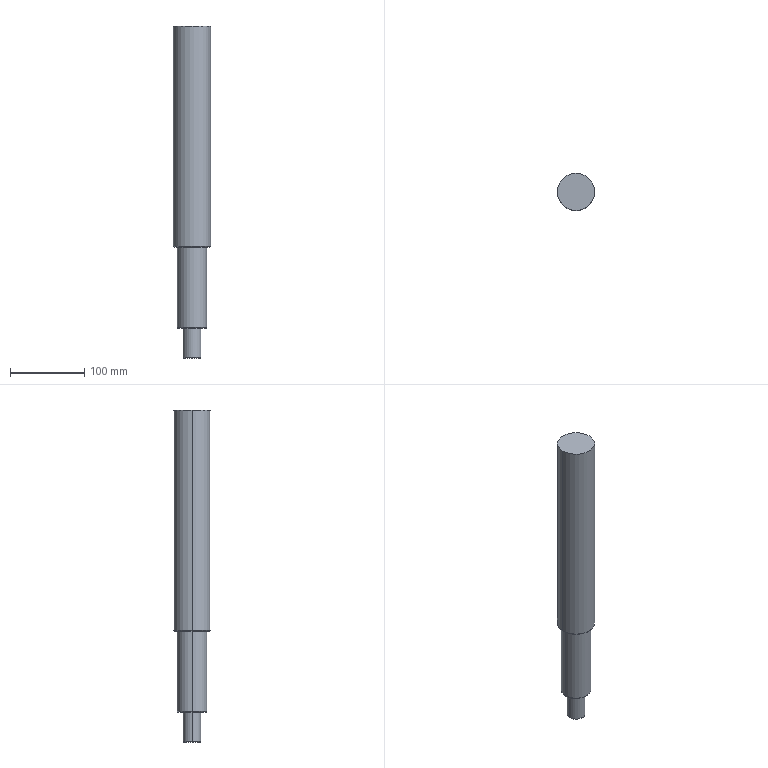Part | SolidWorks | features ICE 2, Chamfer 1, Extrusion 1 | 1 solid | 16 faces | box 50 x 50 x 446 mm | volume 738051 mm3 | cone 6 | cylinder 6 | plane 4 | commonest cylinder face diameters 24 x2 40 x2 50 x2
STEP:
#1=CARTESIAN_POINT('',(-24.,0.,-197.));
#2=VERTEX_POINT('',#1);
#3=CARTESIAN_POINT('',(24.,0.,-197.));
#4=VERTEX_POINT('',#3);
#5=CARTESIAN_POINT('',(0.,0.,-197.));
#6=DIRECTION('',(0.,0.,-1.));
#7=DIRECTION('',(-1.,0.,0.));
#8=AXIS2_PLACEMENT_3D('',#5,#6,#7);
#9=CIRCLE('',#8,24.);
#10=EDGE_CURVE('',#2,#4,#9,.T.);
#11=ORIENTED_EDGE('',*,*,#10,.F.);
#12=CARTESIAN_POINT('',(-25.,0.,-196.));
#13=VERTEX_POINT('',#12);
#14=CARTESIAN_POINT('',(-24.,0.,-197.));
#15=DIRECTION('',(-0.7071,0.,0.7071));
#16=VECTOR('',#15,1000.);
#17=LINE('',#14,#16);
#18=EDGE_CURVE('',#2,#13,#17,.T.);
#19=ORIENTED_EDGE('',*,*,#18,.T.);
#20=CARTESIAN_POINT('',(25.,0.,-196.));
#21=VERTEX_POINT('',#20);
#22=CARTESIAN_POINT('',(0.,0.,-196.));
#23=DIRECTION('',(0.,0.,1.));
#24=DIRECTION('',(-1.,0.,0.));
#25=AXIS2_PLACEMENT_3D('',#22,#23,#24);
#26=CIRCLE('',#25,25.);
#27=EDGE_CURVE('',#21,#13,#26,.T.);
#28=ORIENTED_EDGE('',*,*,#27,.F.);
#29=CARTESIAN_POINT('',(24.,0.,-197.));
#30=DIRECTION('',(0.7071,0.,0.7071));
#31=VECTOR('',#30,1000.);
#32=LINE('',#29,#31);
#33=EDGE_CURVE('',#4,#21,#32,.T.);
#34=ORIENTED_EDGE('',*,*,#33,.F.);
#35=EDGE_LOOP('',(#11,#19,#28,#34));
#36=FACE_OUTER_BOUND('',#35,.T.);
#37=CARTESIAN_POINT('',(0.,0.,-197.));
#38=DIRECTION('',(0.,0.,1.));
#39=DIRECTION('',(1.,0.,0.));
#40=AXIS2_PLACEMENT_3D('',#37,#38,#39);
#41=CONICAL_SURFACE('',#40,24.,0.7854);
#42=ADVANCED_FACE('',(#36),#41,.T.);
#43=CARTESIAN_POINT('',(-19.,0.,-306.));
#44=VERTEX_POINT('',#43);
#45=CARTESIAN_POINT('',(19.,0.,-306.));
#46=VERTEX_POINT('',#45);
#47=CARTESIAN_POINT('',(0.,0.,-306.));
#48=DIRECTION('',(0.,0.,-1.));
#49=DIRECTION('',(-1.,0.,0.));
#50=AXIS2_PLACEMENT_3D('',#47,#48,#49);
#51=CIRCLE('',#50,19.);
#52=EDGE_CURVE('',#44,#46,#51,.T.);
#53=ORIENTED_EDGE('',*,*,#52,.F.);
#54=CARTESIAN_POINT('',(-20.,0.,-305.));
#55=VERTEX_POINT('',#54);
#56=CARTESIAN_POINT('',(-20.,0.,-305.));
#57=DIRECTION('',(-0.7071,0.,0.7071));
#58=VECTOR('',#57,1000.);
#59=LINE('',#56,#58);
#60=EDGE_CURVE('',#44,#55,#59,.T.);
#61=ORIENTED_EDGE('',*,*,#60,.T.);
#62=CARTESIAN_POINT('',(20.,0.,-305.));
#63=VERTEX_POINT('',#62);
#64=CARTESIAN_POINT('',(0.,0.,-305.));
#65=DIRECTION('',(0.,0.,1.));
#66=DIRECTION('',(-1.,0.,0.));
#67=AXIS2_PLACEMENT_3D('',#64,#65,#66);
#68=CIRCLE('',#67,20.);
#69=EDGE_CURVE('',#63,#55,#68,.T.);
#70=ORIENTED_EDGE('',*,*,#69,.F.);
#71=CARTESIAN_POINT('',(20.,0.,-305.));
#72=DIRECTION('',(0.7071,0.,0.7071));
#73=VECTOR('',#72,1000.);
#74=LINE('',#71,#73);
#75=EDGE_CURVE('',#46,#63,#74,.T.);
#76=ORIENTED_EDGE('',*,*,#75,.F.);
#77=EDGE_LOOP('',(#53,#61,#70,#76));
#78=FACE_OUTER_BOUND('',#77,.T.);
#79=CARTESIAN_POINT('',(0.,0.,-305.));
#80=DIRECTION('',(0.,0.,1.));
#81=DIRECTION('',(1.,0.,0.));
#82=AXIS2_PLACEMENT_3D('',#79,#80,#81);
#83=CONICAL_SURFACE('',#82,20.,0.7854);
#84=ADVANCED_FACE('',(#78),#83,.T.);
#85=CARTESIAN_POINT('',(-11.,0.,-346.));
#86=VERTEX_POINT('',#85);
#87=CARTESIAN_POINT('',(11.,0.,-346.));
#88=VERTEX_POINT('',#87);
#89=CARTESIAN_POINT('',(0.,0.,-346.));
#90=DIRECTION('',(0.,0.,-1.));
#91=DIRECTION('',(1.,0.,0.));
#92=AXIS2_PLACEMENT_3D('',#89,#90,#91);
#93=CIRCLE('',#92,11.);
#94=EDGE_CURVE('',#86,#88,#93,.T.);
#95=ORIENTED_EDGE('',*,*,#94,.F.);
#96=CARTESIAN_POINT('',(-12.,0.,-345.));
#97=VERTEX_POINT('',#96);
#98=CARTESIAN_POINT('',(-11.,0.,-346.));
#99=DIRECTION('',(-0.7071,0.,0.7071));
#100=VECTOR('',#99,1000.);
#101=LINE('',#98,#100);
#102=EDGE_CURVE('',#86,#97,#101,.T.);
#103=ORIENTED_EDGE('',*,*,#102,.T.);
#104=CARTESIAN_POINT('',(12.,0.,-345.));
#105=VERTEX_POINT('',#104);
#106=CARTESIAN_POINT('',(0.,0.,-345.));
#107=DIRECTION('',(0.,0.,1.));
#108=DIRECTION('',(1.,0.,0.));
#109=AXIS2_PLACEMENT_3D('',#106,#107,#108);
#110=CIRCLE('',#109,12.);
#111=EDGE_CURVE('',#105,#97,#110,.T.);
#112=ORIENTED_EDGE('',*,*,#111,.F.);
#113=CARTESIAN_POINT('',(11.,0.,-346.));
#114=DIRECTION('',(0.7071,0.,0.7071));
#115=VECTOR('',#114,1000.);
#116=LINE('',#113,#115);
#117=EDGE_CURVE('',#88,#105,#116,.T.);
#118=ORIENTED_EDGE('',*,*,#117,.F.);
#119=EDGE_LOOP('',(#95,#103,#112,#118));
#120=FACE_OUTER_BOUND('',#119,.T.);
#121=CARTESIAN_POINT('',(0.,0.,-346.));
#122=DIRECTION('',(0.,0.,1.));
#123=DIRECTION('',(1.,0.,0.));
#124=AXIS2_PLACEMENT_3D('',#121,#122,#123);
#125=CONICAL_SURFACE('',#124,11.,0.7854);
#126=ADVANCED_FACE('',(#120),#125,.T.);
#127=CARTESIAN_POINT('',(-12.,0.,-306.));
#128=VERTEX_POINT('',#127);
#129=CARTESIAN_POINT('',(12.,0.,-306.));
#130=VERTEX_POINT('',#129);
#131=CARTESIAN_POINT('',(0.,0.,-306.));
#132=DIRECTION('',(0.,0.,-1.));
#133=DIRECTION('',(-1.,0.,0.));
#134=AXIS2_PLACEMENT_3D('',#131,#132,#133);
#135=CIRCLE('',#134,12.);
#136=EDGE_CURVE('',#128,#130,#135,.T.);
#137=ORIENTED_EDGE('',*,*,#136,.T.);
#138=CARTESIAN_POINT('',(12.,0.,-306.));
#139=DIRECTION('',(0.,0.,-1.));
#140=VECTOR('',#139,1000.);
#141=LINE('',#138,#140);
#142=EDGE_CURVE('',#130,#105,#141,.T.);
#143=ORIENTED_EDGE('',*,*,#142,.T.);
#144=ORIENTED_EDGE('',*,*,#111,.T.);
#145=CARTESIAN_POINT('',(-12.,0.,-306.));
#146=DIRECTION('',(0.,0.,-1.));
#147=VECTOR('',#146,1000.);
#148=LINE('',#145,#147);
#149=EDGE_CURVE('',#128,#97,#148,.T.);
#150=ORIENTED_EDGE('',*,*,#149,.F.);
#151=EDGE_LOOP('',(#137,#143,#144,#150));
#152=FACE_OUTER_BOUND('',#151,.T.);
#153=CARTESIAN_POINT('',(0.,0.,-306.));
#154=DIRECTION('',(0.,0.,-1.));
#155=DIRECTION('',(-1.,0.,0.));
#156=AXIS2_PLACEMENT_3D('',#153,#154,#155);
#157=CYLINDRICAL_SURFACE('',#156,12.);
#158=ADVANCED_FACE('',(#152),#157,.T.);
#159=CARTESIAN_POINT('',(-20.,0.,-197.));
#160=VERTEX_POINT('',#159);
#161=CARTESIAN_POINT('',(20.,0.,-197.));
#162=VERTEX_POINT('',#161);
#163=CARTESIAN_POINT('',(0.,0.,-197.));
#164=DIRECTION('',(0.,0.,-1.));
#165=DIRECTION('',(-1.,0.,0.));
#166=AXIS2_PLACEMENT_3D('',#163,#164,#165);
#167=CIRCLE('',#166,20.);
#168=EDGE_CURVE('',#160,#162,#167,.T.);
#169=ORIENTED_EDGE('',*,*,#168,.T.);
#170=CARTESIAN_POINT('',(20.,0.,-197.));
#171=DIRECTION('',(0.,0.,-1.));
#172=VECTOR('',#171,1000.);
#173=LINE('',#170,#172);
#174=EDGE_CURVE('',#162,#63,#173,.T.);
#175=ORIENTED_EDGE('',*,*,#174,.T.);
#176=ORIENTED_EDGE('',*,*,#69,.T.);
#177=CARTESIAN_POINT('',(-20.,0.,-197.));
#178=DIRECTION('',(0.,0.,-1.));
#179=VECTOR('',#178,1000.);
#180=LINE('',#177,#179);
#181=EDGE_CURVE('',#160,#55,#180,.T.);
#182=ORIENTED_EDGE('',*,*,#181,.F.);
#183=EDGE_LOOP('',(#169,#175,#176,#182));
#184=FACE_OUTER_BOUND('',#183,.T.);
#185=CARTESIAN_POINT('',(0.,0.,-197.));
#186=DIRECTION('',(0.,0.,-1.));
#187=DIRECTION('',(-1.,0.,0.));
#188=AXIS2_PLACEMENT_3D('',#185,#186,#187);
#189=CYLINDRICAL_SURFACE('',#188,20.);
#190=ADVANCED_FACE('',(#184),#189,.T.);
#191=ORIENTED_EDGE('',*,*,#27,.T.);
#192=CARTESIAN_POINT('',(-25.,0.,100.));
#193=VERTEX_POINT('',#192);
#194=CARTESIAN_POINT('',(-25.,0.,-346.));
#195=DIRECTION('',(0.,0.,1.));
#196=VECTOR('',#195,1000.);
#197=LINE('',#194,#196);
#198=EDGE_CURVE('',#13,#193,#197,.T.);
#199=ORIENTED_EDGE('',*,*,#198,.T.);
#200=CARTESIAN_POINT('',(25.,0.,100.));
#201=VERTEX_POINT('',#200);
#202=CARTESIAN_POINT('',(0.,0.,100.));
#203=DIRECTION('',(0.,0.,1.));
#204=DIRECTION('',(1.,0.,0.));
#205=AXIS2_PLACEMENT_3D('',#202,#203,#204);
#206=CIRCLE('',#205,25.);
#207=EDGE_CURVE('',#201,#193,#206,.T.);
#208=ORIENTED_EDGE('',*,*,#207,.F.);
#209=CARTESIAN_POINT('',(25.,0.,-346.));
#210=DIRECTION('',(0.,0.,1.));
#211=VECTOR('',#210,1000.);
#212=LINE('',#209,#211);
#213=EDGE_CURVE('',#21,#201,#212,.T.);
#214=ORIENTED_EDGE('',*,*,#213,.F.);
#215=EDGE_LOOP('',(#191,#199,#208,#214));
#216=FACE_OUTER_BOUND('',#215,.T.);
#217=CARTESIAN_POINT('',(0.,0.,-346.));
#218=DIRECTION('',(0.,0.,1.));
#219=DIRECTION('',(1.,0.,0.));
#220=AXIS2_PLACEMENT_3D('',#217,#218,#219);
#221=CYLINDRICAL_SURFACE('',#220,25.);
#222=ADVANCED_FACE('',(#216),#221,.T.);
#223=ORIENTED_EDGE('',*,*,#198,.F.);
#224=CARTESIAN_POINT('',(0.,0.,-196.));
#225=DIRECTION('',(0.,0.,1.));
#226=DIRECTION('',(-1.,0.,0.));
#227=AXIS2_PLACEMENT_3D('',#224,#225,#226);
#228=CIRCLE('',#227,25.);
#229=EDGE_CURVE('',#13,#21,#228,.T.);
#230=ORIENTED_EDGE('',*,*,#229,.T.);
#231=ORIENTED_EDGE('',*,*,#213,.T.);
#232=CARTESIAN_POINT('',(0.,0.,100.));
#233=DIRECTION('',(0.,0.,1.));
#234=DIRECTION('',(1.,0.,0.));
#235=AXIS2_PLACEMENT_3D('',#232,#233,#234);
#236=CIRCLE('',#235,25.);
#237=EDGE_CURVE('',#193,#201,#236,.T.);
#238=ORIENTED_EDGE('',*,*,#237,.F.);
#239=EDGE_LOOP('',(#223,#230,#231,#238));
#240=FACE_OUTER_BOUND('',#239,.T.);
#241=CARTESIAN_POINT('',(0.,0.,-346.));
#242=DIRECTION('',(0.,0.,1.));
#243=DIRECTION('',(1.,0.,0.));
#244=AXIS2_PLACEMENT_3D('',#241,#242,#243);
#245=CYLINDRICAL_SURFACE('',#244,25.);
#246=ADVANCED_FACE('',(#240),#245,.T.);
#247=ORIENTED_EDGE('',*,*,#207,.T.);
#248=ORIENTED_EDGE('',*,*,#237,.T.);
#249=EDGE_LOOP('',(#247,#248));
#250=FACE_OUTER_BOUND('',#249,.T.);
#251=CARTESIAN_POINT('',(0.,0.,100.));
#252=DIRECTION('',(0.,0.,1.));
#253=DIRECTION('',(1.,0.,0.));
#254=AXIS2_PLACEMENT_3D('',#251,#252,#253);
#255=PLANE('',#254);
#256=ADVANCED_FACE('',(#250),#255,.T.);
#257=CARTESIAN_POINT('',(0.,0.,-197.));
#258=DIRECTION('',(0.,0.,-1.));
#259=DIRECTION('',(-1.,0.,0.));
#260=AXIS2_PLACEMENT_3D('',#257,#258,#259);
#261=CIRCLE('',#260,24.);
#262=EDGE_CURVE('',#4,#2,#261,.T.);
#263=ORIENTED_EDGE('',*,*,#262,.T.);
#264=ORIENTED_EDGE('',*,*,#10,.T.);
#265=EDGE_LOOP('',(#263,#264));
#266=FACE_OUTER_BOUND('',#265,.T.);
#267=ORIENTED_EDGE('',*,*,#168,.F.);
#268=CARTESIAN_POINT('',(0.,0.,-197.));
#269=DIRECTION('',(0.,0.,-1.));
#270=DIRECTION('',(-1.,0.,0.));
#271=AXIS2_PLACEMENT_3D('',#268,#269,#270);
#272=CIRCLE('',#271,20.);
#273=EDGE_CURVE('',#162,#160,#272,.T.);
#274=ORIENTED_EDGE('',*,*,#273,.F.);
#275=EDGE_LOOP('',(#267,#274));
#276=FACE_BOUND('',#275,.T.);
#277=CARTESIAN_POINT('',(0.,0.,-197.));
#278=DIRECTION('',(0.,0.,-1.));
#279=DIRECTION('',(-1.,0.,0.));
#280=AXIS2_PLACEMENT_3D('',#277,#278,#279);
#281=PLANE('',#280);
#282=ADVANCED_FACE('',(#266,#276),#281,.T.);
#283=ORIENTED_EDGE('',*,*,#174,.F.);
#284=ORIENTED_EDGE('',*,*,#273,.T.);
#285=ORIENTED_EDGE('',*,*,#181,.T.);
#286=CARTESIAN_POINT('',(0.,0.,-305.));
#287=DIRECTION('',(0.,0.,1.));
#288=DIRECTION('',(-1.,0.,0.));
#289=AXIS2_PLACEMENT_3D('',#286,#287,#288);
#290=CIRCLE('',#289,20.);
#291=EDGE_CURVE('',#55,#63,#290,.T.);
#292=ORIENTED_EDGE('',*,*,#291,.T.);
#293=EDGE_LOOP('',(#283,#284,#285,#292));
#294=FACE_OUTER_BOUND('',#293,.T.);
#295=CARTESIAN_POINT('',(0.,0.,-197.));
#296=DIRECTION('',(0.,0.,-1.));
#297=DIRECTION('',(-1.,0.,0.));
#298=AXIS2_PLACEMENT_3D('',#295,#296,#297);
#299=CYLINDRICAL_SURFACE('',#298,20.);
#300=ADVANCED_FACE('',(#294),#299,.T.);
#301=CARTESIAN_POINT('',(0.,0.,-306.));
#302=DIRECTION('',(0.,0.,-1.));
#303=DIRECTION('',(-1.,0.,0.));
#304=AXIS2_PLACEMENT_3D('',#301,#302,#303);
#305=CIRCLE('',#304,19.);
#306=EDGE_CURVE('',#46,#44,#305,.T.);
#307=ORIENTED_EDGE('',*,*,#306,.T.);
#308=ORIENTED_EDGE('',*,*,#52,.T.);
#309=EDGE_LOOP('',(#307,#308));
#310=FACE_OUTER_BOUND('',#309,.T.);
#311=ORIENTED_EDGE('',*,*,#136,.F.);
#312=CARTESIAN_POINT('',(0.,0.,-306.));
#313=DIRECTION('',(0.,0.,-1.));
#314=DIRECTION('',(-1.,0.,0.));
#315=AXIS2_PLACEMENT_3D('',#312,#313,#314);
#316=CIRCLE('',#315,12.);
#317=EDGE_CURVE('',#130,#128,#316,.T.);
#318=ORIENTED_EDGE('',*,*,#317,.F.);
#319=EDGE_LOOP('',(#311,#318));
#320=FACE_BOUND('',#319,.T.);
#321=CARTESIAN_POINT('',(0.,0.,-306.));
#322=DIRECTION('',(0.,0.,-1.));
#323=DIRECTION('',(-1.,0.,0.));
#324=AXIS2_PLACEMENT_3D('',#321,#322,#323);
#325=PLANE('',#324);
#326=ADVANCED_FACE('',(#310,#320),#325,.T.);
#327=ORIENTED_EDGE('',*,*,#142,.F.);
#328=ORIENTED_EDGE('',*,*,#317,.T.);
#329=ORIENTED_EDGE('',*,*,#149,.T.);
#330=CARTESIAN_POINT('',(0.,0.,-345.));
#331=DIRECTION('',(0.,0.,1.));
#332=DIRECTION('',(1.,0.,0.));
#333=AXIS2_PLACEMENT_3D('',#330,#331,#332);
#334=CIRCLE('',#333,12.);
#335=EDGE_CURVE('',#97,#105,#334,.T.);
#336=ORIENTED_EDGE('',*,*,#335,.T.);
#337=EDGE_LOOP('',(#327,#328,#329,#336));
#338=FACE_OUTER_BOUND('',#337,.T.);
#339=CARTESIAN_POINT('',(0.,0.,-306.));
#340=DIRECTION('',(0.,0.,-1.));
#341=DIRECTION('',(-1.,0.,0.));
#342=AXIS2_PLACEMENT_3D('',#339,#340,#341);
#343=CYLINDRICAL_SURFACE('',#342,12.);
#344=ADVANCED_FACE('',(#338),#343,.T.);
#345=CARTESIAN_POINT('',(0.,0.,-346.));
#346=DIRECTION('',(0.,0.,-1.));
#347=DIRECTION('',(1.,0.,0.));
#348=AXIS2_PLACEMENT_3D('',#345,#346,#347);
#349=CIRCLE('',#348,11.);
#350=EDGE_CURVE('',#88,#86,#349,.T.);
#351=ORIENTED_EDGE('',*,*,#350,.T.);
#352=ORIENTED_EDGE('',*,*,#94,.T.);
#353=EDGE_LOOP('',(#351,#352));
#354=FACE_OUTER_BOUND('',#353,.T.);
#355=CARTESIAN_POINT('',(0.,0.,-346.));
#356=DIRECTION('',(0.,0.,1.));
#357=DIRECTION('',(1.,0.,0.));
#358=AXIS2_PLACEMENT_3D('',#355,#356,#357);
#359=PLANE('',#358);
#360=ADVANCED_FACE('',(#354),#359,.F.);
#361=ORIENTED_EDGE('',*,*,#102,.F.);
#362=ORIENTED_EDGE('',*,*,#350,.F.);
#363=ORIENTED_EDGE('',*,*,#117,.T.);
#364=ORIENTED_EDGE('',*,*,#335,.F.);
#365=EDGE_LOOP('',(#361,#362,#363,#364));
#366=FACE_OUTER_BOUND('',#365,.T.);
#367=CARTESIAN_POINT('',(0.,0.,-346.));
#368=DIRECTION('',(0.,0.,1.));
#369=DIRECTION('',(1.,0.,0.));
#370=AXIS2_PLACEMENT_3D('',#367,#368,#369);
#371=CONICAL_SURFACE('',#370,11.,0.7854);
#372=ADVANCED_FACE('',(#366),#371,.T.);
#373=ORIENTED_EDGE('',*,*,#60,.F.);
#374=ORIENTED_EDGE('',*,*,#306,.F.);
#375=ORIENTED_EDGE('',*,*,#75,.T.);
#376=ORIENTED_EDGE('',*,*,#291,.F.);
#377=EDGE_LOOP('',(#373,#374,#375,#376));
#378=FACE_OUTER_BOUND('',#377,.T.);
#379=CARTESIAN_POINT('',(0.,0.,-305.));
#380=DIRECTION('',(0.,0.,1.));
#381=DIRECTION('',(1.,0.,0.));
#382=AXIS2_PLACEMENT_3D('',#379,#380,#381);
#383=CONICAL_SURFACE('',#382,20.,0.7854);
#384=ADVANCED_FACE('',(#378),#383,.T.);
#385=ORIENTED_EDGE('',*,*,#18,.F.);
#386=ORIENTED_EDGE('',*,*,#262,.F.);
#387=ORIENTED_EDGE('',*,*,#33,.T.);
#388=ORIENTED_EDGE('',*,*,#229,.F.);
#389=EDGE_LOOP('',(#385,#386,#387,#388));
#390=FACE_OUTER_BOUND('',#389,.T.);
#391=CARTESIAN_POINT('',(0.,0.,-197.));
#392=DIRECTION('',(0.,0.,1.));
#393=DIRECTION('',(1.,0.,0.));
#394=AXIS2_PLACEMENT_3D('',#391,#392,#393);
#395=CONICAL_SURFACE('',#394,24.,0.7854);
#396=ADVANCED_FACE('',(#390),#395,.T.);
#397=CLOSED_SHELL('',(#42,#84,#126,#158,#190,#222,#246,#256,#282,#300,#326,#344,#360,#372,#384,#396));
#398=MANIFOLD_SOLID_BREP('',#397);
#399=CARTESIAN_POINT('',(0.,0.,0.));
#400=DIRECTION('',(0.,0.,1.));
#401=DIRECTION('',(1.,0.,0.));
#402=AXIS2_PLACEMENT_3D('',#399,#400,#401);
#403=(LENGTH_UNIT()NAMED_UNIT(*)SI_UNIT(.MILLI.,.METRE.));
#404=UNCERTAINTY_MEASURE_WITH_UNIT(LENGTH_MEASURE(0.00001),#403,'','');
#405=(NAMED_UNIT(*)PLANE_ANGLE_UNIT()SI_UNIT($,.RADIAN.));
#406=(NAMED_UNIT(*)SI_UNIT($,.STERADIAN.)SOLID_ANGLE_UNIT());
#407=(GEOMETRIC_REPRESENTATION_CONTEXT(3)GLOBAL_UNCERTAINTY_ASSIGNED_CONTEXT((#404))GLOBAL_UNIT_ASSIGNED_CONTEXT((#403,#405,#406))REPRESENTATION_CONTEXT('',''));
#408=ADVANCED_BREP_SHAPE_REPRESENTATION('',(#398,#402),#407);